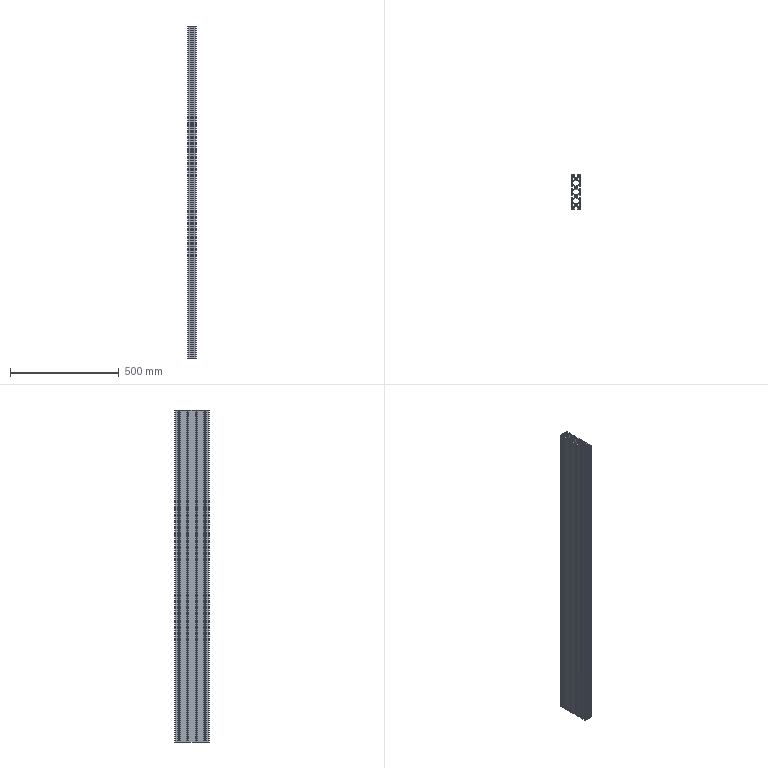Part | STEP file | 0245_022_HFS8-40160-1530-LCH-RCH | 1 solid | 472 faces | box 40 x 160 x 1530 mm | volume 3125718 mm3 | cylinder 252 | plane 220 | commonest cylinder face diameters 0.8 x88 2 x64 10.5 x44 8 x32 0.6 x20 6 x4